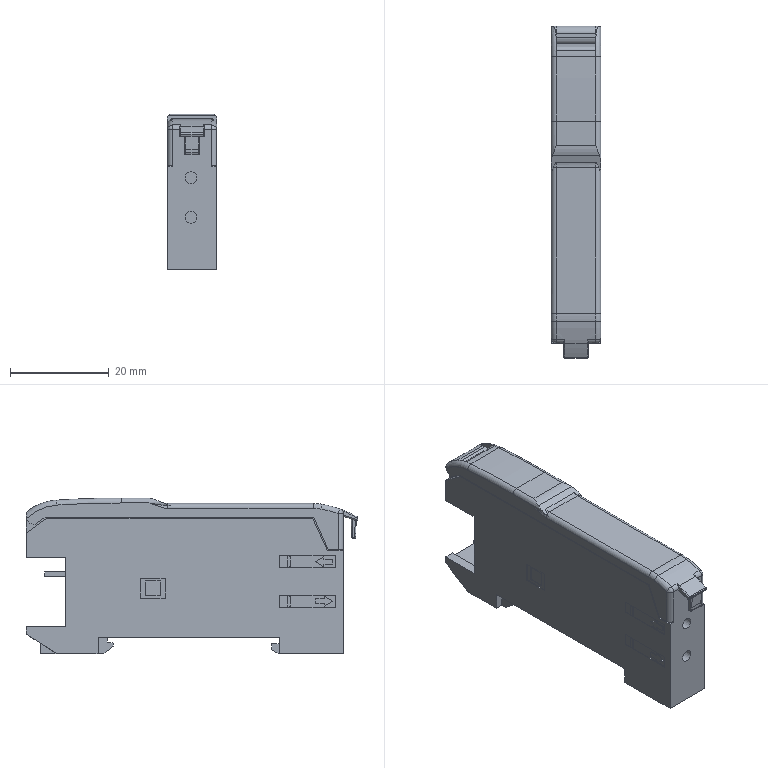Part | NX | features 5003_104_Fiber amplifier 2 | 1 solid | 217 faces | box 10.028 x 67.3 x 31.605 mm | volume 16919 mm3 | plane 147 | cylinder 43 | torus 18 | spline 7 | sphere 2 | commonest cylinder face diameters 0.4 x16 2 x9 3.2 x5 0.6 x4 2.4 x2 19.91 x2